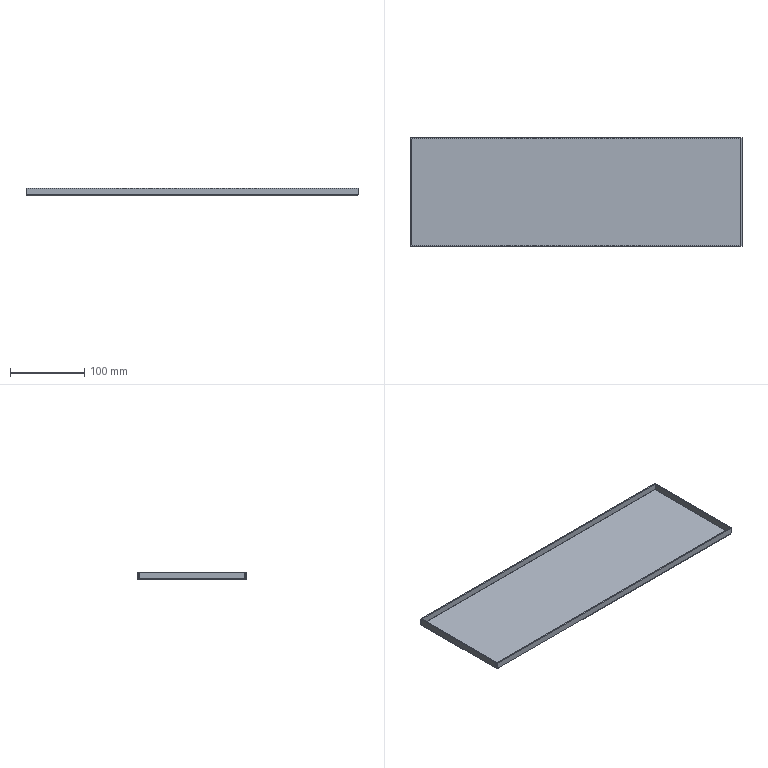Part | SolidWorks | features BaseBody 1 | 1 solid | 38 faces | box 446 x 146 x 10 mm | volume 111927 mm3 | plane 30 | cylinder 8 | commonest cylinder face diameters 0.4 x4 3.4 x4
STEP:
#1=CARTESIAN_POINT('',(1251.5,567.,426.7));
#2=VERTEX_POINT('',#1);
#3=CARTESIAN_POINT('',(1251.3,567.,426.5));
#4=VERTEX_POINT('',#3);
#5=CARTESIAN_POINT('',(1251.3,567.,426.7));
#6=DIRECTION('',(0.,1.,0.));
#7=DIRECTION('',(-1.,0.,0.));
#8=AXIS2_PLACEMENT_3D('',#5,#6,#7);
#9=CIRCLE('',#8,0.2);
#10=EDGE_CURVE('',#2,#4,#9,.T.);
#11=ORIENTED_EDGE('',*,*,#10,.F.);
#12=CARTESIAN_POINT('',(1251.5,709.,426.7));
#13=VERTEX_POINT('',#12);
#14=CARTESIAN_POINT('',(1251.5,567.,426.7));
#15=DIRECTION('',(0.,-1.,0.));
#16=VECTOR('',#15,1000.);
#17=LINE('',#14,#16);
#18=EDGE_CURVE('',#13,#2,#17,.T.);
#19=ORIENTED_EDGE('',*,*,#18,.F.);
#20=CARTESIAN_POINT('',(1251.3,709.,426.5));
#21=VERTEX_POINT('',#20);
#22=CARTESIAN_POINT('',(1251.3,709.,426.7));
#23=DIRECTION('',(0.,-1.,0.));
#24=DIRECTION('',(-1.,0.,0.));
#25=AXIS2_PLACEMENT_3D('',#22,#23,#24);
#26=CIRCLE('',#25,0.2);
#27=EDGE_CURVE('',#21,#13,#26,.T.);
#28=ORIENTED_EDGE('',*,*,#27,.F.);
#29=CARTESIAN_POINT('',(1251.3,567.,426.5));
#30=DIRECTION('',(0.,1.,0.));
#31=VECTOR('',#30,1000.);
#32=LINE('',#29,#31);
#33=EDGE_CURVE('',#4,#21,#32,.T.);
#34=ORIENTED_EDGE('',*,*,#33,.F.);
#35=EDGE_LOOP('',(#11,#19,#28,#34));
#36=FACE_OUTER_BOUND('',#35,.T.);
#37=CARTESIAN_POINT('',(1251.3,90.52,426.7));
#38=DIRECTION('',(0.,1.,0.));
#39=DIRECTION('',(-1.,0.,0.));
#40=AXIS2_PLACEMENT_3D('',#37,#38,#39);
#41=CYLINDRICAL_SURFACE('',#40,0.2);
#42=ADVANCED_FACE('',(#36),#41,.F.);
#43=CARTESIAN_POINT('',(1253.,567.,426.7));
#44=VERTEX_POINT('',#43);
#45=CARTESIAN_POINT('',(1251.3,567.,425.));
#46=VERTEX_POINT('',#45);
#47=CARTESIAN_POINT('',(1251.3,567.,426.7));
#48=DIRECTION('',(0.,1.,0.));
#49=DIRECTION('',(-1.,0.,0.));
#50=AXIS2_PLACEMENT_3D('',#47,#48,#49);
#51=CIRCLE('',#50,1.7);
#52=EDGE_CURVE('',#44,#46,#51,.T.);
#53=ORIENTED_EDGE('',*,*,#52,.T.);
#54=CARTESIAN_POINT('',(1251.3,709.,425.));
#55=VERTEX_POINT('',#54);
#56=CARTESIAN_POINT('',(1251.3,567.,425.));
#57=DIRECTION('',(0.,1.,0.));
#58=VECTOR('',#57,1000.);
#59=LINE('',#56,#58);
#60=EDGE_CURVE('',#46,#55,#59,.T.);
#61=ORIENTED_EDGE('',*,*,#60,.T.);
#62=CARTESIAN_POINT('',(1253.,709.,426.7));
#63=VERTEX_POINT('',#62);
#64=CARTESIAN_POINT('',(1251.3,709.,426.7));
#65=DIRECTION('',(0.,-1.,0.));
#66=DIRECTION('',(-1.,0.,0.));
#67=AXIS2_PLACEMENT_3D('',#64,#65,#66);
#68=CIRCLE('',#67,1.7);
#69=EDGE_CURVE('',#55,#63,#68,.T.);
#70=ORIENTED_EDGE('',*,*,#69,.T.);
#71=CARTESIAN_POINT('',(1253.,567.,426.7));
#72=DIRECTION('',(0.,-1.,0.));
#73=VECTOR('',#72,1000.);
#74=LINE('',#71,#73);
#75=EDGE_CURVE('',#63,#44,#74,.T.);
#76=ORIENTED_EDGE('',*,*,#75,.T.);
#77=EDGE_LOOP('',(#53,#61,#70,#76));
#78=FACE_OUTER_BOUND('',#77,.T.);
#79=CARTESIAN_POINT('',(1251.3,90.52,426.7));
#80=DIRECTION('',(0.,1.,0.));
#81=DIRECTION('',(-1.,0.,0.));
#82=AXIS2_PLACEMENT_3D('',#79,#80,#81);
#83=CYLINDRICAL_SURFACE('',#82,1.7);
#84=ADVANCED_FACE('',(#78),#83,.T.);
#85=CARTESIAN_POINT('',(809.,566.5,426.7));
#86=VERTEX_POINT('',#85);
#87=CARTESIAN_POINT('',(809.,566.7,426.5));
#88=VERTEX_POINT('',#87);
#89=CARTESIAN_POINT('',(809.,566.7,426.7));
#90=DIRECTION('',(1.,0.,0.));
#91=DIRECTION('',(0.,0.,-1.));
#92=AXIS2_PLACEMENT_3D('',#89,#90,#91);
#93=CIRCLE('',#92,0.2);
#94=EDGE_CURVE('',#86,#88,#93,.T.);
#95=ORIENTED_EDGE('',*,*,#94,.F.);
#96=CARTESIAN_POINT('',(1251.,566.5,426.7));
#97=VERTEX_POINT('',#96);
#98=CARTESIAN_POINT('',(809.,566.5,426.7));
#99=DIRECTION('',(-1.,0.,0.));
#100=VECTOR('',#99,1000.);
#101=LINE('',#98,#100);
#102=EDGE_CURVE('',#97,#86,#101,.T.);
#103=ORIENTED_EDGE('',*,*,#102,.F.);
#104=CARTESIAN_POINT('',(1251.,566.7,426.5));
#105=VERTEX_POINT('',#104);
#106=CARTESIAN_POINT('',(1251.,566.7,426.7));
#107=DIRECTION('',(-1.,0.,0.));
#108=DIRECTION('',(0.,0.,-1.));
#109=AXIS2_PLACEMENT_3D('',#106,#107,#108);
#110=CIRCLE('',#109,0.2);
#111=EDGE_CURVE('',#105,#97,#110,.T.);
#112=ORIENTED_EDGE('',*,*,#111,.F.);
#113=CARTESIAN_POINT('',(809.,566.7,426.5));
#114=DIRECTION('',(1.,0.,0.));
#115=VECTOR('',#114,1000.);
#116=LINE('',#113,#115);
#117=EDGE_CURVE('',#88,#105,#116,.T.);
#118=ORIENTED_EDGE('',*,*,#117,.F.);
#119=EDGE_LOOP('',(#95,#103,#112,#118));
#120=FACE_OUTER_BOUND('',#119,.T.);
#121=CARTESIAN_POINT('',(330.185,566.7,426.7));
#122=DIRECTION('',(1.,0.,0.));
#123=DIRECTION('',(0.,0.,-1.));
#124=AXIS2_PLACEMENT_3D('',#121,#122,#123);
#125=CYLINDRICAL_SURFACE('',#124,0.2);
#126=ADVANCED_FACE('',(#120),#125,.F.);
#127=CARTESIAN_POINT('',(809.,565.,426.7));
#128=VERTEX_POINT('',#127);
#129=CARTESIAN_POINT('',(809.,566.7,425.));
#130=VERTEX_POINT('',#129);
#131=CARTESIAN_POINT('',(809.,566.7,426.7));
#132=DIRECTION('',(1.,0.,0.));
#133=DIRECTION('',(0.,0.,-1.));
#134=AXIS2_PLACEMENT_3D('',#131,#132,#133);
#135=CIRCLE('',#134,1.7);
#136=EDGE_CURVE('',#128,#130,#135,.T.);
#137=ORIENTED_EDGE('',*,*,#136,.T.);
#138=CARTESIAN_POINT('',(1251.,566.7,425.));
#139=VERTEX_POINT('',#138);
#140=CARTESIAN_POINT('',(809.,566.7,425.));
#141=DIRECTION('',(1.,0.,0.));
#142=VECTOR('',#141,1000.);
#143=LINE('',#140,#142);
#144=EDGE_CURVE('',#130,#139,#143,.T.);
#145=ORIENTED_EDGE('',*,*,#144,.T.);
#146=CARTESIAN_POINT('',(1251.,565.,426.7));
#147=VERTEX_POINT('',#146);
#148=CARTESIAN_POINT('',(1251.,566.7,426.7));
#149=DIRECTION('',(-1.,0.,0.));
#150=DIRECTION('',(0.,0.,-1.));
#151=AXIS2_PLACEMENT_3D('',#148,#149,#150);
#152=CIRCLE('',#151,1.7);
#153=EDGE_CURVE('',#139,#147,#152,.T.);
#154=ORIENTED_EDGE('',*,*,#153,.T.);
#155=CARTESIAN_POINT('',(809.,565.,426.7));
#156=DIRECTION('',(-1.,0.,0.));
#157=VECTOR('',#156,1000.);
#158=LINE('',#155,#157);
#159=EDGE_CURVE('',#147,#128,#158,.T.);
#160=ORIENTED_EDGE('',*,*,#159,.T.);
#161=EDGE_LOOP('',(#137,#145,#154,#160));
#162=FACE_OUTER_BOUND('',#161,.T.);
#163=CARTESIAN_POINT('',(330.185,566.7,426.7));
#164=DIRECTION('',(1.,0.,0.));
#165=DIRECTION('',(0.,0.,-1.));
#166=AXIS2_PLACEMENT_3D('',#163,#164,#165);
#167=CYLINDRICAL_SURFACE('',#166,1.7);
#168=ADVANCED_FACE('',(#162),#167,.T.);
#169=CARTESIAN_POINT('',(808.5,709.,426.7));
#170=VERTEX_POINT('',#169);
#171=CARTESIAN_POINT('',(808.7,709.,426.5));
#172=VERTEX_POINT('',#171);
#173=CARTESIAN_POINT('',(808.7,709.,426.7));
#174=DIRECTION('',(0.,-1.,0.));
#175=DIRECTION('',(1.,0.,0.));
#176=AXIS2_PLACEMENT_3D('',#173,#174,#175);
#177=CIRCLE('',#176,0.2);
#178=EDGE_CURVE('',#170,#172,#177,.T.);
#179=ORIENTED_EDGE('',*,*,#178,.F.);
#180=CARTESIAN_POINT('',(808.5,567.,426.7));
#181=VERTEX_POINT('',#180);
#182=CARTESIAN_POINT('',(808.5,709.,426.7));
#183=DIRECTION('',(0.,1.,0.));
#184=VECTOR('',#183,1000.);
#185=LINE('',#182,#184);
#186=EDGE_CURVE('',#181,#170,#185,.T.);
#187=ORIENTED_EDGE('',*,*,#186,.F.);
#188=CARTESIAN_POINT('',(808.7,567.,426.5));
#189=VERTEX_POINT('',#188);
#190=CARTESIAN_POINT('',(808.7,567.,426.7));
#191=DIRECTION('',(0.,1.,0.));
#192=DIRECTION('',(1.,0.,0.));
#193=AXIS2_PLACEMENT_3D('',#190,#191,#192);
#194=CIRCLE('',#193,0.2);
#195=EDGE_CURVE('',#189,#181,#194,.T.);
#196=ORIENTED_EDGE('',*,*,#195,.F.);
#197=CARTESIAN_POINT('',(808.7,709.,426.5));
#198=DIRECTION('',(0.,-1.,0.));
#199=VECTOR('',#198,1000.);
#200=LINE('',#197,#199);
#201=EDGE_CURVE('',#172,#189,#200,.T.);
#202=ORIENTED_EDGE('',*,*,#201,.F.);
#203=EDGE_LOOP('',(#179,#187,#196,#202));
#204=FACE_OUTER_BOUND('',#203,.T.);
#205=CARTESIAN_POINT('',(808.7,1194.876,426.7));
#206=DIRECTION('',(0.,-1.,0.));
#207=DIRECTION('',(1.,0.,0.));
#208=AXIS2_PLACEMENT_3D('',#205,#206,#207);
#209=CYLINDRICAL_SURFACE('',#208,0.2);
#210=ADVANCED_FACE('',(#204),#209,.F.);
#211=CARTESIAN_POINT('',(807.,709.,426.7));
#212=VERTEX_POINT('',#211);
#213=CARTESIAN_POINT('',(808.7,709.,425.));
#214=VERTEX_POINT('',#213);
#215=CARTESIAN_POINT('',(808.7,709.,426.7));
#216=DIRECTION('',(0.,-1.,0.));
#217=DIRECTION('',(1.,0.,0.));
#218=AXIS2_PLACEMENT_3D('',#215,#216,#217);
#219=CIRCLE('',#218,1.7);
#220=EDGE_CURVE('',#212,#214,#219,.T.);
#221=ORIENTED_EDGE('',*,*,#220,.T.);
#222=CARTESIAN_POINT('',(808.7,567.,425.));
#223=VERTEX_POINT('',#222);
#224=CARTESIAN_POINT('',(808.7,709.,425.));
#225=DIRECTION('',(0.,-1.,0.));
#226=VECTOR('',#225,1000.);
#227=LINE('',#224,#226);
#228=EDGE_CURVE('',#214,#223,#227,.T.);
#229=ORIENTED_EDGE('',*,*,#228,.T.);
#230=CARTESIAN_POINT('',(807.,567.,426.7));
#231=VERTEX_POINT('',#230);
#232=CARTESIAN_POINT('',(808.7,567.,426.7));
#233=DIRECTION('',(0.,1.,0.));
#234=DIRECTION('',(1.,0.,0.));
#235=AXIS2_PLACEMENT_3D('',#232,#233,#234);
#236=CIRCLE('',#235,1.7);
#237=EDGE_CURVE('',#223,#231,#236,.T.);
#238=ORIENTED_EDGE('',*,*,#237,.T.);
#239=CARTESIAN_POINT('',(807.,709.,426.7));
#240=DIRECTION('',(0.,1.,0.));
#241=VECTOR('',#240,1000.);
#242=LINE('',#239,#241);
#243=EDGE_CURVE('',#231,#212,#242,.T.);
#244=ORIENTED_EDGE('',*,*,#243,.T.);
#245=EDGE_LOOP('',(#221,#229,#238,#244));
#246=FACE_OUTER_BOUND('',#245,.T.);
#247=CARTESIAN_POINT('',(808.7,1194.876,426.7));
#248=DIRECTION('',(0.,-1.,0.));
#249=DIRECTION('',(1.,0.,0.));
#250=AXIS2_PLACEMENT_3D('',#247,#248,#249);
#251=CYLINDRICAL_SURFACE('',#250,1.7);
#252=ADVANCED_FACE('',(#246),#251,.T.);
#253=CARTESIAN_POINT('',(1251.,709.5,426.7));
#254=VERTEX_POINT('',#253);
#255=CARTESIAN_POINT('',(1251.,709.3,426.5));
#256=VERTEX_POINT('',#255);
#257=CARTESIAN_POINT('',(1251.,709.3,426.7));
#258=DIRECTION('',(-1.,0.,0.));
#259=DIRECTION('',(0.,0.,1.));
#260=AXIS2_PLACEMENT_3D('',#257,#258,#259);
#261=CIRCLE('',#260,0.2);
#262=EDGE_CURVE('',#254,#256,#261,.T.);
#263=ORIENTED_EDGE('',*,*,#262,.F.);
#264=CARTESIAN_POINT('',(809.,709.5,426.7));
#265=VERTEX_POINT('',#264);
#266=CARTESIAN_POINT('',(1251.,709.5,426.7));
#267=DIRECTION('',(1.,0.,0.));
#268=VECTOR('',#267,1000.);
#269=LINE('',#266,#268);
#270=EDGE_CURVE('',#265,#254,#269,.T.);
#271=ORIENTED_EDGE('',*,*,#270,.F.);
#272=CARTESIAN_POINT('',(809.,709.3,426.5));
#273=VERTEX_POINT('',#272);
#274=CARTESIAN_POINT('',(809.,709.3,426.7));
#275=DIRECTION('',(1.,0.,0.));
#276=DIRECTION('',(0.,0.,1.));
#277=AXIS2_PLACEMENT_3D('',#274,#275,#276);
#278=CIRCLE('',#277,0.2);
#279=EDGE_CURVE('',#273,#265,#278,.T.);
#280=ORIENTED_EDGE('',*,*,#279,.F.);
#281=CARTESIAN_POINT('',(1251.,709.3,426.5));
#282=DIRECTION('',(-1.,0.,0.));
#283=VECTOR('',#282,1000.);
#284=LINE('',#281,#283);
#285=EDGE_CURVE('',#256,#273,#284,.T.);
#286=ORIENTED_EDGE('',*,*,#285,.F.);
#287=EDGE_LOOP('',(#263,#271,#280,#286));
#288=FACE_OUTER_BOUND('',#287,.T.);
#289=CARTESIAN_POINT('',(1739.18,709.3,426.7));
#290=DIRECTION('',(-1.,0.,0.));
#291=DIRECTION('',(0.,0.,1.));
#292=AXIS2_PLACEMENT_3D('',#289,#290,#291);
#293=CYLINDRICAL_SURFACE('',#292,0.2);
#294=ADVANCED_FACE('',(#288),#293,.F.);
#295=CARTESIAN_POINT('',(1251.,711.,426.7));
#296=VERTEX_POINT('',#295);
#297=CARTESIAN_POINT('',(1251.,709.3,425.));
#298=VERTEX_POINT('',#297);
#299=CARTESIAN_POINT('',(1251.,709.3,426.7));
#300=DIRECTION('',(-1.,0.,0.));
#301=DIRECTION('',(0.,0.,1.));
#302=AXIS2_PLACEMENT_3D('',#299,#300,#301);
#303=CIRCLE('',#302,1.7);
#304=EDGE_CURVE('',#296,#298,#303,.T.);
#305=ORIENTED_EDGE('',*,*,#304,.T.);
#306=CARTESIAN_POINT('',(809.,709.3,425.));
#307=VERTEX_POINT('',#306);
#308=CARTESIAN_POINT('',(1251.,709.3,425.));
#309=DIRECTION('',(-1.,0.,0.));
#310=VECTOR('',#309,1000.);
#311=LINE('',#308,#310);
#312=EDGE_CURVE('',#298,#307,#311,.T.);
#313=ORIENTED_EDGE('',*,*,#312,.T.);
#314=CARTESIAN_POINT('',(809.,711.,426.7));
#315=VERTEX_POINT('',#314);
#316=CARTESIAN_POINT('',(809.,709.3,426.7));
#317=DIRECTION('',(1.,0.,0.));
#318=DIRECTION('',(0.,0.,1.));
#319=AXIS2_PLACEMENT_3D('',#316,#317,#318);
#320=CIRCLE('',#319,1.7);
#321=EDGE_CURVE('',#307,#315,#320,.T.);
#322=ORIENTED_EDGE('',*,*,#321,.T.);
#323=CARTESIAN_POINT('',(1251.,711.,426.7));
#324=DIRECTION('',(1.,0.,0.));
#325=VECTOR('',#324,1000.);
#326=LINE('',#323,#325);
#327=EDGE_CURVE('',#315,#296,#326,.T.);
#328=ORIENTED_EDGE('',*,*,#327,.T.);
#329=EDGE_LOOP('',(#305,#313,#322,#328));
#330=FACE_OUTER_BOUND('',#329,.T.);
#331=CARTESIAN_POINT('',(1739.18,709.3,426.7));
#332=DIRECTION('',(-1.,0.,0.));
#333=DIRECTION('',(0.,0.,1.));
#334=AXIS2_PLACEMENT_3D('',#331,#332,#333);
#335=CYLINDRICAL_SURFACE('',#334,1.7);
#336=ADVANCED_FACE('',(#330),#335,.T.);
#337=CARTESIAN_POINT('',(1251.,709.,426.5));
#338=VERTEX_POINT('',#337);
#339=CARTESIAN_POINT('',(1251.,0.,426.5));
#340=DIRECTION('',(0.,1.,0.));
#341=VECTOR('',#340,1000.);
#342=LINE('',#339,#341);
#343=EDGE_CURVE('',#338,#256,#342,.T.);
#344=ORIENTED_EDGE('',*,*,#343,.T.);
#345=ORIENTED_EDGE('',*,*,#285,.T.);
#346=CARTESIAN_POINT('',(809.,709.,426.5));
#347=VERTEX_POINT('',#346);
#348=CARTESIAN_POINT('',(809.,0.,426.5));
#349=DIRECTION('',(0.,-1.,0.));
#350=VECTOR('',#349,1000.);
#351=LINE('',#348,#350);
#352=EDGE_CURVE('',#273,#347,#351,.T.);
#353=ORIENTED_EDGE('',*,*,#352,.T.);
#354=CARTESIAN_POINT('',(0.,709.,426.5));
#355=DIRECTION('',(-1.,0.,0.));
#356=VECTOR('',#355,1000.);
#357=LINE('',#354,#356);
#358=EDGE_CURVE('',#347,#172,#357,.T.);
#359=ORIENTED_EDGE('',*,*,#358,.T.);
#360=ORIENTED_EDGE('',*,*,#201,.T.);
#361=CARTESIAN_POINT('',(809.,567.,426.5));
#362=VERTEX_POINT('',#361);
#363=CARTESIAN_POINT('',(0.,567.,426.5));
#364=DIRECTION('',(1.,0.,0.));
#365=VECTOR('',#364,1000.);
#366=LINE('',#363,#365);
#367=EDGE_CURVE('',#189,#362,#366,.T.);
#368=ORIENTED_EDGE('',*,*,#367,.T.);
#369=CARTESIAN_POINT('',(809.,0.,426.5));
#370=DIRECTION('',(0.,-1.,0.));
#371=VECTOR('',#370,1000.);
#372=LINE('',#369,#371);
#373=EDGE_CURVE('',#362,#88,#372,.T.);
#374=ORIENTED_EDGE('',*,*,#373,.T.);
#375=ORIENTED_EDGE('',*,*,#117,.T.);
#376=CARTESIAN_POINT('',(1251.,567.,426.5));
#377=VERTEX_POINT('',#376);
#378=CARTESIAN_POINT('',(1251.,0.,426.5));
#379=DIRECTION('',(0.,1.,0.));
#380=VECTOR('',#379,1000.);
#381=LINE('',#378,#380);
#382=EDGE_CURVE('',#105,#377,#381,.T.);
#383=ORIENTED_EDGE('',*,*,#382,.T.);
#384=CARTESIAN_POINT('',(0.,567.,426.5));
#385=DIRECTION('',(1.,0.,0.));
#386=VECTOR('',#385,1000.);
#387=LINE('',#384,#386);
#388=EDGE_CURVE('',#377,#4,#387,.T.);
#389=ORIENTED_EDGE('',*,*,#388,.T.);
#390=ORIENTED_EDGE('',*,*,#33,.T.);
#391=CARTESIAN_POINT('',(0.,709.,426.5));
#392=DIRECTION('',(-1.,0.,0.));
#393=VECTOR('',#392,1000.);
#394=LINE('',#391,#393);
#395=EDGE_CURVE('',#21,#338,#394,.T.);
#396=ORIENTED_EDGE('',*,*,#395,.T.);
#397=EDGE_LOOP('',(#344,#345,#353,#359,#360,#368,#374,#375,#383,#389,#390,#396));
#398=FACE_OUTER_BOUND('',#397,.T.);
#399=CARTESIAN_POINT('',(0.,0.,426.5));
#400=DIRECTION('',(0.,0.,1.));
#401=DIRECTION('',(1.,0.,0.));
#402=AXIS2_PLACEMENT_3D('',#399,#400,#401);
#403=PLANE('',#402);
#404=ADVANCED_FACE('',(#398),#403,.T.);
#405=ORIENTED_EDGE('',*,*,#382,.F.);
#406=ORIENTED_EDGE('',*,*,#111,.T.);
#407=CARTESIAN_POINT('',(1251.,1458.654,426.7));
#408=DIRECTION('',(0.,-1.,0.));
#409=VECTOR('',#408,1000.);
#410=LINE('',#407,#409);
#411=EDGE_CURVE('',#97,#147,#410,.T.);
#412=ORIENTED_EDGE('',*,*,#411,.T.);
#413=ORIENTED_EDGE('',*,*,#153,.F.);
#414=CARTESIAN_POINT('',(1251.,567.,425.));
#415=VERTEX_POINT('',#414);
#416=CARTESIAN_POINT('',(1251.,0.,425.));
#417=DIRECTION('',(0.,1.,0.));
#418=VECTOR('',#417,1000.);
#419=LINE('',#416,#418);
#420=EDGE_CURVE('',#139,#415,#419,.T.);
#421=ORIENTED_EDGE('',*,*,#420,.T.);
#422=CARTESIAN_POINT('',(1251.,567.,1356.51));
#423=DIRECTION('',(0.,0.,-1.));
#424=VECTOR('',#423,1000.);
#425=LINE('',#422,#424);
#426=EDGE_CURVE('',#377,#415,#425,.T.);
#427=ORIENTED_EDGE('',*,*,#426,.F.);
#428=EDGE_LOOP('',(#405,#406,#412,#413,#421,#427));
#429=FACE_OUTER_BOUND('',#428,.T.);
#430=CARTESIAN_POINT('',(1251.,0.,1356.51));
#431=DIRECTION('',(-1.,0.,0.));
#432=DIRECTION('',(0.,1.,0.));
#433=AXIS2_PLACEMENT_3D('',#430,#431,#432);
#434=PLANE('',#433);
#435=ADVANCED_FACE('',(#429),#434,.F.);
#436=CARTESIAN_POINT('',(809.,567.,425.));
#437=VERTEX_POINT('',#436);
#438=CARTESIAN_POINT('',(809.,567.,1356.51));
#439=DIRECTION('',(0.,0.,-1.));
#440=VECTOR('',#439,1000.);
#441=LINE('',#438,#440);
#442=EDGE_CURVE('',#362,#437,#441,.T.);
#443=ORIENTED_EDGE('',*,*,#442,.T.);
#444=CARTESIAN_POINT('',(809.,0.,425.));
#445=DIRECTION('',(0.,-1.,0.));
#446=VECTOR('',#445,1000.);
#447=LINE('',#444,#446);
#448=EDGE_CURVE('',#437,#130,#447,.T.);
#449=ORIENTED_EDGE('',*,*,#448,.T.);
#450=ORIENTED_EDGE('',*,*,#136,.F.);
#451=CARTESIAN_POINT('',(809.,1458.654,426.7));
#452=DIRECTION('',(0.,-1.,0.));
#453=VECTOR('',#452,1000.);
#454=LINE('',#451,#453);
#455=EDGE_CURVE('',#86,#128,#454,.T.);
#456=ORIENTED_EDGE('',*,*,#455,.F.);
#457=ORIENTED_EDGE('',*,*,#94,.T.);
#458=ORIENTED_EDGE('',*,*,#373,.F.);
#459=EDGE_LOOP('',(#443,#449,#450,#456,#457,#458));
#460=FACE_OUTER_BOUND('',#459,.T.);
#461=CARTESIAN_POINT('',(809.,0.,1356.51));
#462=DIRECTION('',(1.,0.,0.));
#463=DIRECTION('',(0.,0.,-1.));
#464=AXIS2_PLACEMENT_3D('',#461,#462,#463);
#465=PLANE('',#464);
#466=ADVANCED_FACE('',(#460),#465,.F.);
#467=ORIENTED_EDGE('',*,*,#352,.F.);
#468=ORIENTED_EDGE('',*,*,#279,.T.);
#469=CARTESIAN_POINT('',(809.,-182.654,426.7));
#470=DIRECTION('',(0.,1.,0.));
#471=VECTOR('',#470,1000.);
#472=LINE('',#469,#471);
#473=EDGE_CURVE('',#265,#315,#472,.T.);
#474=ORIENTED_EDGE('',*,*,#473,.T.);
#475=ORIENTED_EDGE('',*,*,#321,.F.);
#476=CARTESIAN_POINT('',(809.,709.,425.));
#477=VERTEX_POINT('',#476);
#478=CARTESIAN_POINT('',(809.,0.,425.));
#479=DIRECTION('',(0.,-1.,0.));
#480=VECTOR('',#479,1000.);
#481=LINE('',#478,#480);
#482=EDGE_CURVE('',#307,#477,#481,.T.);
#483=ORIENTED_EDGE('',*,*,#482,.T.);
#484=CARTESIAN_POINT('',(809.,709.,1356.51));
#485=DIRECTION('',(0.,0.,-1.));
#486=VECTOR('',#485,1000.);
#487=LINE('',#484,#486);
#488=EDGE_CURVE('',#347,#477,#487,.T.);
#489=ORIENTED_EDGE('',*,*,#488,.F.);
#490=EDGE_LOOP('',(#467,#468,#474,#475,#483,#489));
#491=FACE_OUTER_BOUND('',#490,.T.);
#492=CARTESIAN_POINT('',(809.,0.,1356.51));
#493=DIRECTION('',(1.,0.,0.));
#494=DIRECTION('',(0.,0.,-1.));
#495=AXIS2_PLACEMENT_3D('',#492,#493,#494);
#496=PLANE('',#495);
#497=ADVANCED_FACE('',(#491),#496,.F.);
#498=CARTESIAN_POINT('',(1251.,709.,425.));
#499=VERTEX_POINT('',#498);
#500=CARTESIAN_POINT('',(1251.,709.,1356.51));
#501=DIRECTION('',(0.,0.,-1.));
#502=VECTOR('',#501,1000.);
#503=LINE('',#500,#502);
#504=EDGE_CURVE('',#338,#499,#503,.T.);
#505=ORIENTED_EDGE('',*,*,#504,.T.);
#506=CARTESIAN_POINT('',(1251.,0.,425.));
#507=DIRECTION('',(0.,1.,0.));
#508=VECTOR('',#507,1000.);
#509=LINE('',#506,#508);
#510=EDGE_CURVE('',#499,#298,#509,.T.);
#511=ORIENTED_EDGE('',*,*,#510,.T.);
#512=ORIENTED_EDGE('',*,*,#304,.F.);
#513=CARTESIAN_POINT('',(1251.,-182.654,426.7));
#514=DIRECTION('',(0.,1.,0.));
#515=VECTOR('',#514,1000.);
#516=LINE('',#513,#515);
#517=EDGE_CURVE('',#254,#296,#516,.T.);
#518=ORIENTED_EDGE('',*,*,#517,.F.);
#519=ORIENTED_EDGE('',*,*,#262,.T.);
#520=ORIENTED_EDGE('',*,*,#343,.F.);
#521=EDGE_LOOP('',(#505,#511,#512,#518,#519,#520));
#522=FACE_OUTER_BOUND('',#521,.T.);
#523=CARTESIAN_POINT('',(1251.,0.,1356.51));
#524=DIRECTION('',(-1.,0.,0.));
#525=DIRECTION('',(0.,1.,0.));
#526=AXIS2_PLACEMENT_3D('',#523,#524,#525);
#527=PLANE('',#526);
#528=ADVANCED_FACE('',(#522),#527,.F.);
#529=ORIENTED_EDGE('',*,*,#312,.F.);
#530=ORIENTED_EDGE('',*,*,#510,.F.);
#531=CARTESIAN_POINT('',(0.,709.,425.));
#532=DIRECTION('',(-1.,0.,0.));
#533=VECTOR('',#532,1000.);
#534=LINE('',#531,#533);
#535=EDGE_CURVE('',#55,#499,#534,.T.);
#536=ORIENTED_EDGE('',*,*,#535,.F.);
#537=ORIENTED_EDGE('',*,*,#60,.F.);
#538=CARTESIAN_POINT('',(0.,567.,425.));
#539=DIRECTION('',(1.,0.,0.));
#540=VECTOR('',#539,1000.);
#541=LINE('',#538,#540);
#542=EDGE_CURVE('',#415,#46,#541,.T.);
#543=ORIENTED_EDGE('',*,*,#542,.F.);
#544=ORIENTED_EDGE('',*,*,#420,.F.);
#545=ORIENTED_EDGE('',*,*,#144,.F.);
#546=ORIENTED_EDGE('',*,*,#448,.F.);
#547=CARTESIAN_POINT('',(0.,567.,425.));
#548=DIRECTION('',(1.,0.,0.));
#549=VECTOR('',#548,1000.);
#550=LINE('',#547,#549);
#551=EDGE_CURVE('',#223,#437,#550,.T.);
#552=ORIENTED_EDGE('',*,*,#551,.F.);
#553=ORIENTED_EDGE('',*,*,#228,.F.);
#554=CARTESIAN_POINT('',(0.,709.,425.));
#555=DIRECTION('',(-1.,0.,0.));
#556=VECTOR('',#555,1000.);
#557=LINE('',#554,#556);
#558=EDGE_CURVE('',#477,#214,#557,.T.);
#559=ORIENTED_EDGE('',*,*,#558,.F.);
#560=ORIENTED_EDGE('',*,*,#482,.F.);
#561=EDGE_LOOP('',(#529,#530,#536,#537,#543,#544,#545,#546,#552,#553,#559,#560));
#562=FACE_OUTER_BOUND('',#561,.T.);
#563=CARTESIAN_POINT('',(0.,0.,425.));
#564=DIRECTION('',(0.,0.,1.));
#565=DIRECTION('',(1.,0.,0.));
#566=AXIS2_PLACEMENT_3D('',#563,#564,#565);
#567=PLANE('',#566);
#568=ADVANCED_FACE('',(#562),#567,.F.);
#569=CARTESIAN_POINT('',(1253.,709.5,435.));
#570=VERTEX_POINT('',#569);
#571=CARTESIAN_POINT('',(807.,709.5,435.));
#572=VERTEX_POINT('',#571);
#573=CARTESIAN_POINT('',(1251.5,709.5,435.));
#574=DIRECTION('',(-1.,0.,0.));
#575=VECTOR('',#574,1000.);
#576=LINE('',#573,#575);
#577=EDGE_CURVE('',#570,#572,#576,.T.);
#578=ORIENTED_EDGE('',*,*,#577,.T.);
#579=CARTESIAN_POINT('',(807.,709.5,426.7));
#580=VERTEX_POINT('',#579);
#581=CARTESIAN_POINT('',(807.,709.5,-40.508));
#582=DIRECTION('',(0.,0.,-1.));
#583=VECTOR('',#582,1000.);
#584=LINE('',#581,#583);
#585=EDGE_CURVE('',#572,#580,#584,.T.);
#586=ORIENTED_EDGE('',*,*,#585,.T.);
#587=CARTESIAN_POINT('',(806.998,709.5,426.7));
#588=DIRECTION('',(1.,0.,0.));
#589=VECTOR('',#588,1000.);
#590=LINE('',#587,#589);
#591=EDGE_CURVE('',#580,#265,#590,.T.);
#592=ORIENTED_EDGE('',*,*,#591,.T.);
#593=ORIENTED_EDGE('',*,*,#270,.T.);
#594=CARTESIAN_POINT('',(1253.,709.5,426.7));
#595=VERTEX_POINT('',#594);
#596=CARTESIAN_POINT('',(1253.002,709.5,426.7));
#597=DIRECTION('',(-1.,0.,0.));
#598=VECTOR('',#597,1000.);
#599=LINE('',#596,#598);
#600=EDGE_CURVE('',#595,#254,#599,.T.);
#601=ORIENTED_EDGE('',*,*,#600,.F.);
#602=CARTESIAN_POINT('',(1253.,709.5,-40.508));
#603=DIRECTION('',(0.,0.,1.));
#604=VECTOR('',#603,1000.);
#605=LINE('',#602,#604);
#606=EDGE_CURVE('',#595,#570,#605,.T.);
#607=ORIENTED_EDGE('',*,*,#606,.T.);
#608=EDGE_LOOP('',(#578,#586,#592,#593,#601,#607));
#609=FACE_OUTER_BOUND('',#608,.T.);
#610=CARTESIAN_POINT('',(1251.5,709.5,-40.508));
#611=DIRECTION('',(0.,1.,0.));
#612=DIRECTION('',(1.,0.,0.));
#613=AXIS2_PLACEMENT_3D('',#610,#611,#612);
#614=PLANE('',#613);
#615=ADVANCED_FACE('',(#609),#614,.F.);
#616=CARTESIAN_POINT('',(807.,711.,426.7));
#617=VERTEX_POINT('',#616);
#618=CARTESIAN_POINT('',(806.998,711.,426.7));
#619=DIRECTION('',(1.,0.,0.));
#620=VECTOR('',#619,1000.);
#621=LINE('',#618,#620);
#622=EDGE_CURVE('',#617,#315,#621,.T.);
#623=ORIENTED_EDGE('',*,*,#622,.T.);
#624=ORIENTED_EDGE('',*,*,#473,.F.);
#625=ORIENTED_EDGE('',*,*,#591,.F.);
#626=CARTESIAN_POINT('',(807.,-182.654,426.7));
#627=DIRECTION('',(0.,1.,0.));
#628=VECTOR('',#627,1000.);
#629=LINE('',#626,#628);
#630=EDGE_CURVE('',#580,#617,#629,.T.);
#631=ORIENTED_EDGE('',*,*,#630,.T.);
#632=EDGE_LOOP('',(#623,#624,#625,#631));
#633=FACE_OUTER_BOUND('',#632,.T.);
#634=CARTESIAN_POINT('',(806.998,-182.654,426.7));
#635=DIRECTION('',(0.,0.,1.));
#636=DIRECTION('',(1.,0.,0.));
#637=AXIS2_PLACEMENT_3D('',#634,#635,#636);
#638=PLANE('',#637);
#639=ADVANCED_FACE('',(#633),#638,.F.);
#640=ORIENTED_EDGE('',*,*,#327,.F.);
#641=ORIENTED_EDGE('',*,*,#622,.F.);
#642=CARTESIAN_POINT('',(807.,711.,435.));
#643=VERTEX_POINT('',#642);
#644=CARTESIAN_POINT('',(807.,711.,-40.508));
#645=DIRECTION('',(0.,0.,1.));
#646=VECTOR('',#645,1000.);
#647=LINE('',#644,#646);
#648=EDGE_CURVE('',#617,#643,#647,.T.);
#649=ORIENTED_EDGE('',*,*,#648,.T.);
#650=CARTESIAN_POINT('',(1253.,711.,435.));
#651=VERTEX_POINT('',#650);
#652=CARTESIAN_POINT('',(1253.,711.,435.));
#653=DIRECTION('',(1.,0.,0.));
#654=VECTOR('',#653,1000.);
#655=LINE('',#652,#654);
#656=EDGE_CURVE('',#643,#651,#655,.T.);
#657=ORIENTED_EDGE('',*,*,#656,.T.);
#658=CARTESIAN_POINT('',(1253.,711.,426.7));
#659=VERTEX_POINT('',#658);
#660=CARTESIAN_POINT('',(1253.,711.,423.672));
#661=DIRECTION('',(0.,0.,1.));
#662=VECTOR('',#661,1000.);
#663=LINE('',#660,#662);
#664=EDGE_CURVE('',#659,#651,#663,.T.);
#665=ORIENTED_EDGE('',*,*,#664,.F.);
#666=CARTESIAN_POINT('',(1253.002,711.,426.7));
#667=DIRECTION('',(-1.,0.,0.));
#668=VECTOR('',#667,1000.);
#669=LINE('',#666,#668);
#670=EDGE_CURVE('',#659,#296,#669,.T.);
#671=ORIENTED_EDGE('',*,*,#670,.T.);
#672=EDGE_LOOP('',(#640,#641,#649,#657,#665,#671));
#673=FACE_OUTER_BOUND('',#672,.T.);
#674=CARTESIAN_POINT('',(1253.,711.,435.));
#675=DIRECTION('',(0.,1.,0.));
#676=DIRECTION('',(1.,0.,0.));
#677=AXIS2_PLACEMENT_3D('',#674,#675,#676);
#678=PLANE('',#677);
#679=ADVANCED_FACE('',(#673),#678,.T.);
#680=ORIENTED_EDGE('',*,*,#517,.T.);
#681=ORIENTED_EDGE('',*,*,#670,.F.);
#682=CARTESIAN_POINT('',(1253.,-182.654,426.7));
#683=DIRECTION('',(0.,1.,0.));
#684=VECTOR('',#683,1000.);
#685=LINE('',#682,#684);
#686=EDGE_CURVE('',#595,#659,#685,.T.);
#687=ORIENTED_EDGE('',*,*,#686,.F.);
#688=ORIENTED_EDGE('',*,*,#600,.T.);
#689=EDGE_LOOP('',(#680,#681,#687,#688));
#690=FACE_OUTER_BOUND('',#689,.T.);
#691=CARTESIAN_POINT('',(1253.002,-182.654,426.7));
#692=DIRECTION('',(0.,0.,-1.));
#693=DIRECTION('',(-1.,0.,0.));
#694=AXIS2_PLACEMENT_3D('',#691,#692,#693);
#695=PLANE('',#694);
#696=ADVANCED_FACE('',(#690),#695,.T.);
#697=ORIENTED_EDGE('',*,*,#664,.T.);
#698=CARTESIAN_POINT('',(1253.,-182.654,435.));
#699=DIRECTION('',(0.,1.,0.));
#700=VECTOR('',#699,1000.);
#701=LINE('',#698,#700);
#702=EDGE_CURVE('',#570,#651,#701,.T.);
#703=ORIENTED_EDGE('',*,*,#702,.F.);
#704=ORIENTED_EDGE('',*,*,#606,.F.);
#705=ORIENTED_EDGE('',*,*,#686,.T.);
#706=EDGE_LOOP('',(#697,#703,#704,#705));
#707=FACE_OUTER_BOUND('',#706,.T.);
#708=CARTESIAN_POINT('',(1253.,-182.654,-40.508));
#709=DIRECTION('',(-1.,0.,0.));
#710=DIRECTION('',(0.,1.,0.));
#711=AXIS2_PLACEMENT_3D('',#708,#709,#710);
#712=PLANE('',#711);
#713=ADVANCED_FACE('',(#707),#712,.F.);
#714=ORIENTED_EDGE('',*,*,#648,.F.);
#715=ORIENTED_EDGE('',*,*,#630,.F.);
#716=ORIENTED_EDGE('',*,*,#585,.F.);
#717=CARTESIAN_POINT('',(807.,-182.654,435.));
#718=DIRECTION('',(0.,1.,0.));
#719=VECTOR('',#718,1000.);
#720=LINE('',#717,#719);
#721=EDGE_CURVE('',#572,#643,#720,.T.);
#722=ORIENTED_EDGE('',*,*,#721,.T.);
#723=EDGE_LOOP('',(#714,#715,#716,#722));
#724=FACE_OUTER_BOUND('',#723,.T.);
#725=CARTESIAN_POINT('',(807.,-182.654,-40.508));
#726=DIRECTION('',(1.,0.,0.));
#727=DIRECTION('',(0.,0.,-1.));
#728=AXIS2_PLACEMENT_3D('',#725,#726,#727);
#729=PLANE('',#728);
#730=ADVANCED_FACE('',(#724),#729,.F.);
#731=ORIENTED_EDGE('',*,*,#656,.F.);
#732=ORIENTED_EDGE('',*,*,#721,.F.);
#733=ORIENTED_EDGE('',*,*,#577,.F.);
#734=ORIENTED_EDGE('',*,*,#702,.T.);
#735=EDGE_LOOP('',(#731,#732,#733,#734));
#736=FACE_OUTER_BOUND('',#735,.T.);
#737=CARTESIAN_POINT('',(1251.5,-182.654,435.));
#738=DIRECTION('',(0.,0.,-1.));
#739=DIRECTION('',(-1.,0.,0.));
#740=AXIS2_PLACEMENT_3D('',#737,#738,#739);
#741=PLANE('',#740);
#742=ADVANCED_FACE('',(#736),#741,.F.);
#743=CARTESIAN_POINT('',(808.5,567.,435.));
#744=VERTEX_POINT('',#743);
#745=CARTESIAN_POINT('',(808.5,567.,-40.508));
#746=DIRECTION('',(0.,0.,-1.));
#747=VECTOR('',#746,1000.);
#748=LINE('',#745,#747);
#749=EDGE_CURVE('',#744,#181,#748,.T.);
#750=ORIENTED_EDGE('',*,*,#749,.T.);
#751=ORIENTED_EDGE('',*,*,#186,.T.);
#752=CARTESIAN_POINT('',(808.5,709.,435.));
#753=VERTEX_POINT('',#752);
#754=CARTESIAN_POINT('',(808.5,709.,-40.508));
#755=DIRECTION('',(0.,0.,1.));
#756=VECTOR('',#755,1000.);
#757=LINE('',#754,#756);
#758=EDGE_CURVE('',#170,#753,#757,.T.);
#759=ORIENTED_EDGE('',*,*,#758,.T.);
#760=CARTESIAN_POINT('',(808.5,709.5,435.));
#761=DIRECTION('',(0.,-1.,0.));
#762=VECTOR('',#761,1000.);
#763=LINE('',#760,#762);
#764=EDGE_CURVE('',#753,#744,#763,.T.);
#765=ORIENTED_EDGE('',*,*,#764,.T.);
#766=EDGE_LOOP('',(#750,#751,#759,#765));
#767=FACE_OUTER_BOUND('',#766,.T.);
#768=CARTESIAN_POINT('',(808.5,709.5,-40.508));
#769=DIRECTION('',(-1.,0.,0.));
#770=DIRECTION('',(0.,0.,1.));
#771=AXIS2_PLACEMENT_3D('',#768,#769,#770);
#772=PLANE('',#771);
#773=ADVANCED_FACE('',(#767),#772,.F.);
#774=CARTESIAN_POINT('',(807.,567.,435.));
#775=VERTEX_POINT('',#774);
#776=CARTESIAN_POINT('',(807.,567.,-40.508));
#777=DIRECTION('',(0.,0.,1.));
#778=VECTOR('',#777,1000.);
#779=LINE('',#776,#778);
#780=EDGE_CURVE('',#231,#775,#779,.T.);
#781=ORIENTED_EDGE('',*,*,#780,.F.);
#782=ORIENTED_EDGE('',*,*,#237,.F.);
#783=ORIENTED_EDGE('',*,*,#551,.T.);
#784=ORIENTED_EDGE('',*,*,#442,.F.);
#785=ORIENTED_EDGE('',*,*,#367,.F.);
#786=ORIENTED_EDGE('',*,*,#195,.T.);
#787=ORIENTED_EDGE('',*,*,#749,.F.);
#788=CARTESIAN_POINT('',(1092.985,567.,435.));
#789=DIRECTION('',(-1.,0.,0.));
#790=VECTOR('',#789,1000.);
#791=LINE('',#788,#790);
#792=EDGE_CURVE('',#744,#775,#791,.T.);
#793=ORIENTED_EDGE('',*,*,#792,.T.);
#794=EDGE_LOOP('',(#781,#782,#783,#784,#785,#786,#787,#793));
#795=FACE_OUTER_BOUND('',#794,.T.);
#796=CARTESIAN_POINT('',(1092.985,567.,-40.508));
#797=DIRECTION('',(0.,1.,0.));
#798=DIRECTION('',(0.,0.,-1.));
#799=AXIS2_PLACEMENT_3D('',#796,#797,#798);
#800=PLANE('',#799);
#801=ADVANCED_FACE('',(#795),#800,.F.);
#802=ORIENTED_EDGE('',*,*,#243,.F.);
#803=ORIENTED_EDGE('',*,*,#780,.T.);
#804=CARTESIAN_POINT('',(807.,709.,435.));
#805=VERTEX_POINT('',#804);
#806=CARTESIAN_POINT('',(807.,565.,435.));
#807=DIRECTION('',(0.,1.,0.));
#808=VECTOR('',#807,1000.);
#809=LINE('',#806,#808);
#810=EDGE_CURVE('',#775,#805,#809,.T.);
#811=ORIENTED_EDGE('',*,*,#810,.T.);
#812=CARTESIAN_POINT('',(807.,709.,423.672));
#813=DIRECTION('',(0.,0.,1.));
#814=VECTOR('',#813,1000.);
#815=LINE('',#812,#814);
#816=EDGE_CURVE('',#212,#805,#815,.T.);
#817=ORIENTED_EDGE('',*,*,#816,.F.);
#818=EDGE_LOOP('',(#802,#803,#811,#817));
#819=FACE_OUTER_BOUND('',#818,.T.);
#820=CARTESIAN_POINT('',(807.,565.,435.));
#821=DIRECTION('',(-1.,0.,0.));
#822=DIRECTION('',(0.,1.,0.));
#823=AXIS2_PLACEMENT_3D('',#820,#821,#822);
#824=PLANE('',#823);
#825=ADVANCED_FACE('',(#819),#824,.T.);
#826=ORIENTED_EDGE('',*,*,#816,.T.);
#827=CARTESIAN_POINT('',(1092.985,709.,435.));
#828=DIRECTION('',(-1.,0.,0.));
#829=VECTOR('',#828,1000.);
#830=LINE('',#827,#829);
#831=EDGE_CURVE('',#753,#805,#830,.T.);
#832=ORIENTED_EDGE('',*,*,#831,.F.);
#833=ORIENTED_EDGE('',*,*,#758,.F.);
#834=ORIENTED_EDGE('',*,*,#178,.T.);
#835=ORIENTED_EDGE('',*,*,#358,.F.);
#836=ORIENTED_EDGE('',*,*,#488,.T.);
#837=ORIENTED_EDGE('',*,*,#558,.T.);
#838=ORIENTED_EDGE('',*,*,#220,.F.);
#839=EDGE_LOOP('',(#826,#832,#833,#834,#835,#836,#837,#838));
#840=FACE_OUTER_BOUND('',#839,.T.);
#841=CARTESIAN_POINT('',(1092.985,709.,-40.508));
#842=DIRECTION('',(0.,-1.,0.));
#843=DIRECTION('',(0.,0.,-1.));
#844=AXIS2_PLACEMENT_3D('',#841,#842,#843);
#845=PLANE('',#844);
#846=ADVANCED_FACE('',(#840),#845,.F.);
#847=ORIENTED_EDGE('',*,*,#810,.F.);
#848=ORIENTED_EDGE('',*,*,#792,.F.);
#849=ORIENTED_EDGE('',*,*,#764,.F.);
#850=ORIENTED_EDGE('',*,*,#831,.T.);
#851=EDGE_LOOP('',(#847,#848,#849,#850));
#852=FACE_OUTER_BOUND('',#851,.T.);
#853=CARTESIAN_POINT('',(1092.985,709.5,435.));
#854=DIRECTION('',(0.,0.,-1.));
#855=DIRECTION('',(-1.,0.,0.));
#856=AXIS2_PLACEMENT_3D('',#853,#854,#855);
#857=PLANE('',#856);
#858=ADVANCED_FACE('',(#852),#857,.F.);
#859=CARTESIAN_POINT('',(807.,566.5,435.));
#860=VERTEX_POINT('',#859);
#861=CARTESIAN_POINT('',(1253.,566.5,435.));
#862=VERTEX_POINT('',#861);
#863=CARTESIAN_POINT('',(808.5,566.5,435.));
#864=DIRECTION('',(1.,0.,0.));
#865=VECTOR('',#864,1000.);
#866=LINE('',#863,#865);
#867=EDGE_CURVE('',#860,#862,#866,.T.);
#868=ORIENTED_EDGE('',*,*,#867,.T.);
#869=CARTESIAN_POINT('',(1253.,566.5,426.7));
#870=VERTEX_POINT('',#869);
#871=CARTESIAN_POINT('',(1253.,566.5,-40.508));
#872=DIRECTION('',(0.,0.,-1.));
#873=VECTOR('',#872,1000.);
#874=LINE('',#871,#873);
#875=EDGE_CURVE('',#862,#870,#874,.T.);
#876=ORIENTED_EDGE('',*,*,#875,.T.);
#877=CARTESIAN_POINT('',(1253.002,566.5,426.7));
#878=DIRECTION('',(-1.,0.,0.));
#879=VECTOR('',#878,1000.);
#880=LINE('',#877,#879);
#881=EDGE_CURVE('',#870,#97,#880,.T.);
#882=ORIENTED_EDGE('',*,*,#881,.T.);
#883=ORIENTED_EDGE('',*,*,#102,.T.);
#884=CARTESIAN_POINT('',(807.,566.5,426.7));
#885=VERTEX_POINT('',#884);
#886=CARTESIAN_POINT('',(806.998,566.5,426.7));
#887=DIRECTION('',(1.,0.,0.));
#888=VECTOR('',#887,1000.);
#889=LINE('',#886,#888);
#890=EDGE_CURVE('',#885,#86,#889,.T.);
#891=ORIENTED_EDGE('',*,*,#890,.F.);
#892=CARTESIAN_POINT('',(807.,566.5,-40.508));
#893=DIRECTION('',(0.,0.,1.));
#894=VECTOR('',#893,1000.);
#895=LINE('',#892,#894);
#896=EDGE_CURVE('',#885,#860,#895,.T.);
#897=ORIENTED_EDGE('',*,*,#896,.T.);
#898=EDGE_LOOP('',(#868,#876,#882,#883,#891,#897));
#899=FACE_OUTER_BOUND('',#898,.T.);
#900=CARTESIAN_POINT('',(808.5,566.5,-40.508));
#901=DIRECTION('',(0.,-1.,0.));
#902=DIRECTION('',(-1.,0.,0.));
#903=AXIS2_PLACEMENT_3D('',#900,#901,#902);
#904=PLANE('',#903);
#905=ADVANCED_FACE('',(#899),#904,.F.);
#906=CARTESIAN_POINT('',(1253.,565.,426.7));
#907=VERTEX_POINT('',#906);
#908=CARTESIAN_POINT('',(1253.002,565.,426.7));
#909=DIRECTION('',(-1.,0.,0.));
#910=VECTOR('',#909,1000.);
#911=LINE('',#908,#910);
#912=EDGE_CURVE('',#907,#147,#911,.T.);
#913=ORIENTED_EDGE('',*,*,#912,.T.);
#914=ORIENTED_EDGE('',*,*,#411,.F.);
#915=ORIENTED_EDGE('',*,*,#881,.F.);
#916=CARTESIAN_POINT('',(1253.,1458.654,426.7));
#917=DIRECTION('',(0.,-1.,0.));
#918=VECTOR('',#917,1000.);
#919=LINE('',#916,#918);
#920=EDGE_CURVE('',#870,#907,#919,.T.);
#921=ORIENTED_EDGE('',*,*,#920,.T.);
#922=EDGE_LOOP('',(#913,#914,#915,#921));
#923=FACE_OUTER_BOUND('',#922,.T.);
#924=CARTESIAN_POINT('',(1253.002,1458.654,426.7));
#925=DIRECTION('',(0.,0.,1.));
#926=DIRECTION('',(1.,0.,0.));
#927=AXIS2_PLACEMENT_3D('',#924,#925,#926);
#928=PLANE('',#927);
#929=ADVANCED_FACE('',(#923),#928,.F.);
#930=ORIENTED_EDGE('',*,*,#159,.F.);
#931=ORIENTED_EDGE('',*,*,#912,.F.);
#932=CARTESIAN_POINT('',(1253.,565.,435.));
#933=VERTEX_POINT('',#932);
#934=CARTESIAN_POINT('',(1253.,565.,-40.508));
#935=DIRECTION('',(0.,0.,1.));
#936=VECTOR('',#935,1000.);
#937=LINE('',#934,#936);
#938=EDGE_CURVE('',#907,#933,#937,.T.);
#939=ORIENTED_EDGE('',*,*,#938,.T.);
#940=CARTESIAN_POINT('',(807.,565.,435.));
#941=VERTEX_POINT('',#940);
#942=CARTESIAN_POINT('',(1253.,565.,435.));
#943=DIRECTION('',(-1.,0.,0.));
#944=VECTOR('',#943,1000.);
#945=LINE('',#942,#944);
#946=EDGE_CURVE('',#933,#941,#945,.T.);
#947=ORIENTED_EDGE('',*,*,#946,.T.);
#948=CARTESIAN_POINT('',(807.,565.,426.7));
#949=VERTEX_POINT('',#948);
#950=CARTESIAN_POINT('',(807.,565.,423.672));
#951=DIRECTION('',(0.,0.,1.));
#952=VECTOR('',#951,1000.);
#953=LINE('',#950,#952);
#954=EDGE_CURVE('',#949,#941,#953,.T.);
#955=ORIENTED_EDGE('',*,*,#954,.F.);
#956=CARTESIAN_POINT('',(806.998,565.,426.7));
#957=DIRECTION('',(1.,0.,0.));
#958=VECTOR('',#957,1000.);
#959=LINE('',#956,#958);
#960=EDGE_CURVE('',#949,#128,#959,.T.);
#961=ORIENTED_EDGE('',*,*,#960,.T.);
#962=EDGE_LOOP('',(#930,#931,#939,#947,#955,#961));
#963=FACE_OUTER_BOUND('',#962,.T.);
#964=CARTESIAN_POINT('',(1253.,565.,435.));
#965=DIRECTION('',(0.,-1.,0.));
#966=DIRECTION('',(-1.,0.,0.));
#967=AXIS2_PLACEMENT_3D('',#964,#965,#966);
#968=PLANE('',#967);
#969=ADVANCED_FACE('',(#963),#968,.T.);
#970=ORIENTED_EDGE('',*,*,#455,.T.);
#971=ORIENTED_EDGE('',*,*,#960,.F.);
#972=CARTESIAN_POINT('',(807.,1458.654,426.7));
#973=DIRECTION('',(0.,-1.,0.));
#974=VECTOR('',#973,1000.);
#975=LINE('',#972,#974);
#976=EDGE_CURVE('',#885,#949,#975,.T.);
#977=ORIENTED_EDGE('',*,*,#976,.F.);
#978=ORIENTED_EDGE('',*,*,#890,.T.);
#979=EDGE_LOOP('',(#970,#971,#977,#978));
#980=FACE_OUTER_BOUND('',#979,.T.);
#981=CARTESIAN_POINT('',(806.998,1458.654,426.7));
#982=DIRECTION('',(0.,0.,-1.));
#983=DIRECTION('',(-1.,0.,0.));
#984=AXIS2_PLACEMENT_3D('',#981,#982,#983);
#985=PLANE('',#984);
#986=ADVANCED_FACE('',(#980),#985,.T.);
#987=ORIENTED_EDGE('',*,*,#954,.T.);
#988=CARTESIAN_POINT('',(807.,1458.654,435.));
#989=DIRECTION('',(0.,-1.,0.));
#990=VECTOR('',#989,1000.);
#991=LINE('',#988,#990);
#992=EDGE_CURVE('',#860,#941,#991,.T.);
#993=ORIENTED_EDGE('',*,*,#992,.F.);
#994=ORIENTED_EDGE('',*,*,#896,.F.);
#995=ORIENTED_EDGE('',*,*,#976,.T.);
#996=EDGE_LOOP('',(#987,#993,#994,#995));
#997=FACE_OUTER_BOUND('',#996,.T.);
#998=CARTESIAN_POINT('',(807.,1458.654,-40.508));
#999=DIRECTION('',(1.,0.,0.));
#1000=DIRECTION('',(0.,0.,-1.));
#1001=AXIS2_PLACEMENT_3D('',#998,#999,#1000);
#1002=PLANE('',#1001);
#1003=ADVANCED_FACE('',(#997),#1002,.F.);
#1004=ORIENTED_EDGE('',*,*,#938,.F.);
#1005=ORIENTED_EDGE('',*,*,#920,.F.);
#1006=ORIENTED_EDGE('',*,*,#875,.F.);
#1007=CARTESIAN_POINT('',(1253.,1458.654,435.));
#1008=DIRECTION('',(0.,-1.,0.));
#1009=VECTOR('',#1008,1000.);
#1010=LINE('',#1007,#1009);
#1011=EDGE_CURVE('',#862,#933,#1010,.T.);
#1012=ORIENTED_EDGE('',*,*,#1011,.T.);
#1013=EDGE_LOOP('',(#1004,#1005,#1006,#1012));
#1014=FACE_OUTER_BOUND('',#1013,.T.);
#1015=CARTESIAN_POINT('',(1253.,1458.654,-40.508));
#1016=DIRECTION('',(-1.,0.,0.));
#1017=DIRECTION('',(0.,1.,0.));
#1018=AXIS2_PLACEMENT_3D('',#1015,#1016,#1017);
#1019=PLANE('',#1018);
#1020=ADVANCED_FACE('',(#1014),#1019,.F.);
#1021=ORIENTED_EDGE('',*,*,#946,.F.);
#1022=ORIENTED_EDGE('',*,*,#1011,.F.);
#1023=ORIENTED_EDGE('',*,*,#867,.F.);
#1024=ORIENTED_EDGE('',*,*,#992,.T.);
#1025=EDGE_LOOP('',(#1021,#1022,#1023,#1024));
#1026=FACE_OUTER_BOUND('',#1025,.T.);
#1027=CARTESIAN_POINT('',(808.5,1458.654,435.));
#1028=DIRECTION('',(0.,0.,-1.));
#1029=DIRECTION('',(-1.,0.,0.));
#1030=AXIS2_PLACEMENT_3D('',#1027,#1028,#1029);
#1031=PLANE('',#1030);
#1032=ADVANCED_FACE('',(#1026),#1031,.F.);
#1033=CARTESIAN_POINT('',(1251.5,709.,435.));
#1034=VERTEX_POINT('',#1033);
#1035=CARTESIAN_POINT('',(1251.5,709.,-40.508));
#1036=DIRECTION('',(0.,0.,-1.));
#1037=VECTOR('',#1036,1000.);
#1038=LINE('',#1035,#1037);
#1039=EDGE_CURVE('',#1034,#13,#1038,.T.);
#1040=ORIENTED_EDGE('',*,*,#1039,.T.);
#1041=ORIENTED_EDGE('',*,*,#18,.T.);
#1042=CARTESIAN_POINT('',(1251.5,567.,435.));
#1043=VERTEX_POINT('',#1042);
#1044=CARTESIAN_POINT('',(1251.5,567.,-40.508));
#1045=DIRECTION('',(0.,0.,1.));
#1046=VECTOR('',#1045,1000.);
#1047=LINE('',#1044,#1046);
#1048=EDGE_CURVE('',#2,#1043,#1047,.T.);
#1049=ORIENTED_EDGE('',*,*,#1048,.T.);
#1050=CARTESIAN_POINT('',(1251.5,566.5,435.));
#1051=DIRECTION('',(0.,1.,0.));
#1052=VECTOR('',#1051,1000.);
#1053=LINE('',#1050,#1052);
#1054=EDGE_CURVE('',#1043,#1034,#1053,.T.);
#1055=ORIENTED_EDGE('',*,*,#1054,.T.);
#1056=EDGE_LOOP('',(#1040,#1041,#1049,#1055));
#1057=FACE_OUTER_BOUND('',#1056,.T.);
#1058=CARTESIAN_POINT('',(1251.5,566.5,-40.508));
#1059=DIRECTION('',(1.,0.,0.));
#1060=DIRECTION('',(0.,-1.,0.));
#1061=AXIS2_PLACEMENT_3D('',#1058,#1059,#1060);
#1062=PLANE('',#1061);
#1063=ADVANCED_FACE('',(#1057),#1062,.F.);
#1064=CARTESIAN_POINT('',(1253.,709.,435.));
#1065=VERTEX_POINT('',#1064);
#1066=CARTESIAN_POINT('',(1253.,709.,-40.508));
#1067=DIRECTION('',(0.,0.,1.));
#1068=VECTOR('',#1067,1000.);
#1069=LINE('',#1066,#1068);
#1070=EDGE_CURVE('',#63,#1065,#1069,.T.);
#1071=ORIENTED_EDGE('',*,*,#1070,.F.);
#1072=ORIENTED_EDGE('',*,*,#69,.F.);
#1073=ORIENTED_EDGE('',*,*,#535,.T.);
#1074=ORIENTED_EDGE('',*,*,#504,.F.);
#1075=ORIENTED_EDGE('',*,*,#395,.F.);
#1076=ORIENTED_EDGE('',*,*,#27,.T.);
#1077=ORIENTED_EDGE('',*,*,#1039,.F.);
#1078=CARTESIAN_POINT('',(967.015,709.,435.));
#1079=DIRECTION('',(1.,0.,0.));
#1080=VECTOR('',#1079,1000.);
#1081=LINE('',#1078,#1080);
#1082=EDGE_CURVE('',#1034,#1065,#1081,.T.);
#1083=ORIENTED_EDGE('',*,*,#1082,.T.);
#1084=EDGE_LOOP('',(#1071,#1072,#1073,#1074,#1075,#1076,#1077,#1083));
#1085=FACE_OUTER_BOUND('',#1084,.T.);
#1086=CARTESIAN_POINT('',(967.015,709.,-40.508));
#1087=DIRECTION('',(0.,-1.,0.));
#1088=DIRECTION('',(-1.,0.,0.));
#1089=AXIS2_PLACEMENT_3D('',#1086,#1087,#1088);
#1090=PLANE('',#1089);
#1091=ADVANCED_FACE('',(#1085),#1090,.F.);
#1092=ORIENTED_EDGE('',*,*,#75,.F.);
#1093=ORIENTED_EDGE('',*,*,#1070,.T.);
#1094=CARTESIAN_POINT('',(1253.,567.,435.));
#1095=VERTEX_POINT('',#1094);
#1096=CARTESIAN_POINT('',(1253.,565.,435.));
#1097=DIRECTION('',(0.,-1.,0.));
#1098=VECTOR('',#1097,1000.);
#1099=LINE('',#1096,#1098);
#1100=EDGE_CURVE('',#1065,#1095,#1099,.T.);
#1101=ORIENTED_EDGE('',*,*,#1100,.T.);
#1102=CARTESIAN_POINT('',(1253.,567.,423.672));
#1103=DIRECTION('',(0.,0.,1.));
#1104=VECTOR('',#1103,1000.);
#1105=LINE('',#1102,#1104);
#1106=EDGE_CURVE('',#44,#1095,#1105,.T.);
#1107=ORIENTED_EDGE('',*,*,#1106,.F.);
#1108=EDGE_LOOP('',(#1092,#1093,#1101,#1107));
#1109=FACE_OUTER_BOUND('',#1108,.T.);
#1110=CARTESIAN_POINT('',(1253.,565.,435.));
#1111=DIRECTION('',(1.,0.,0.));
#1112=DIRECTION('',(0.,0.,-1.));
#1113=AXIS2_PLACEMENT_3D('',#1110,#1111,#1112);
#1114=PLANE('',#1113);
#1115=ADVANCED_FACE('',(#1109),#1114,.T.);
#1116=ORIENTED_EDGE('',*,*,#1106,.T.);
#1117=CARTESIAN_POINT('',(967.015,567.,435.));
#1118=DIRECTION('',(1.,0.,0.));
#1119=VECTOR('',#1118,1000.);
#1120=LINE('',#1117,#1119);
#1121=EDGE_CURVE('',#1043,#1095,#1120,.T.);
#1122=ORIENTED_EDGE('',*,*,#1121,.F.);
#1123=ORIENTED_EDGE('',*,*,#1048,.F.);
#1124=ORIENTED_EDGE('',*,*,#10,.T.);
#1125=ORIENTED_EDGE('',*,*,#388,.F.);
#1126=ORIENTED_EDGE('',*,*,#426,.T.);
#1127=ORIENTED_EDGE('',*,*,#542,.T.);
#1128=ORIENTED_EDGE('',*,*,#52,.F.);
#1129=EDGE_LOOP('',(#1116,#1122,#1123,#1124,#1125,#1126,#1127,#1128));
#1130=FACE_OUTER_BOUND('',#1129,.T.);
#1131=CARTESIAN_POINT('',(967.015,567.,-40.508));
#1132=DIRECTION('',(0.,1.,0.));
#1133=DIRECTION('',(1.,0.,0.));
#1134=AXIS2_PLACEMENT_3D('',#1131,#1132,#1133);
#1135=PLANE('',#1134);
#1136=ADVANCED_FACE('',(#1130),#1135,.F.);
#1137=ORIENTED_EDGE('',*,*,#1100,.F.);
#1138=ORIENTED_EDGE('',*,*,#1082,.F.);
#1139=ORIENTED_EDGE('',*,*,#1054,.F.);
#1140=ORIENTED_EDGE('',*,*,#1121,.T.);
#1141=EDGE_LOOP('',(#1137,#1138,#1139,#1140));
#1142=FACE_OUTER_BOUND('',#1141,.T.);
#1143=CARTESIAN_POINT('',(967.015,566.5,435.));
#1144=DIRECTION('',(0.,0.,-1.));
#1145=DIRECTION('',(0.,-1.,0.));
#1146=AXIS2_PLACEMENT_3D('',#1143,#1144,#1145);
#1147=PLANE('',#1146);
#1148=ADVANCED_FACE('',(#1142),#1147,.F.);
#1149=CLOSED_SHELL('',(#42,#84,#126,#168,#210,#252,#294,#336,#404,#435,#466,#497,#528,#568,#615,#639,#679,#696,#713,#730,#742,#773,#801,#825,#846,#858,#905,#929,#969,#986,#1003,#1020,#1032,#1063,#1091,#1115,#1136,#1148));
#1150=MANIFOLD_SOLID_BREP('',#1149);
#1151=CARTESIAN_POINT('',(0.,0.,0.));
#1152=DIRECTION('',(0.,0.,1.));
#1153=DIRECTION('',(1.,0.,0.));
#1154=AXIS2_PLACEMENT_3D('',#1151,#1152,#1153);
#1155=(LENGTH_UNIT()NAMED_UNIT(*)SI_UNIT(.MILLI.,.METRE.));
#1156=UNCERTAINTY_MEASURE_WITH_UNIT(LENGTH_MEASURE(0.00001),#1155,'','');
#1157=(NAMED_UNIT(*)PLANE_ANGLE_UNIT()SI_UNIT($,.RADIAN.));
#1158=(NAMED_UNIT(*)SI_UNIT($,.STERADIAN.)SOLID_ANGLE_UNIT());
#1159=(GEOMETRIC_REPRESENTATION_CONTEXT(3)GLOBAL_UNCERTAINTY_ASSIGNED_CONTEXT((#1156))GLOBAL_UNIT_ASSIGNED_CONTEXT((#1155,#1157,#1158))REPRESENTATION_CONTEXT('',''));
#1160=ADVANCED_BREP_SHAPE_REPRESENTATION('',(#1150,#1154),#1159);